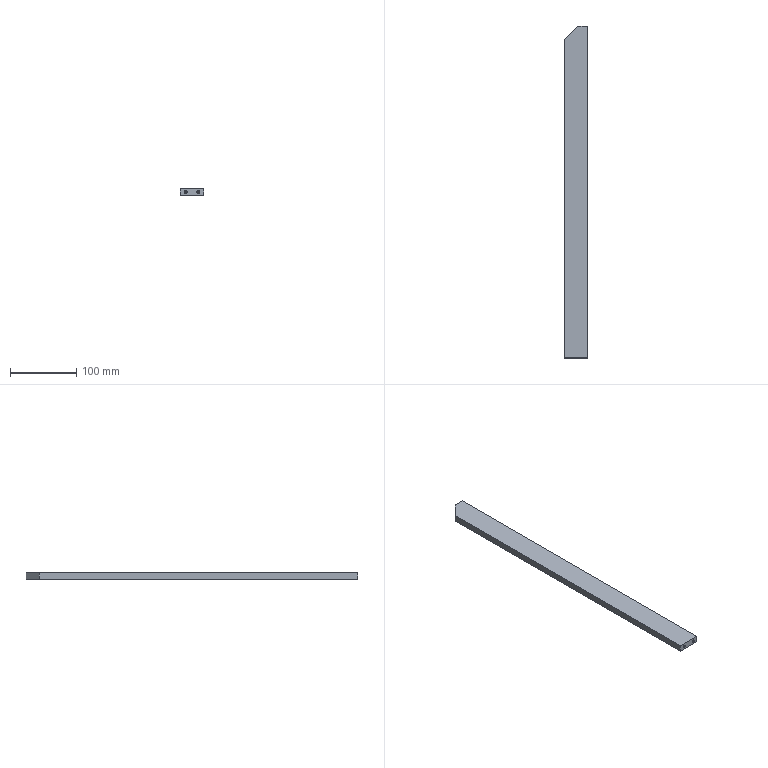Part | STEP file | PN_0035 | 1 solid | 35 faces | box 35 x 500 x 10 mm | volume 171757 mm3 | cylinder 14 | cone 14 | plane 7 | commonest cylinder face diameters 4.2 x14